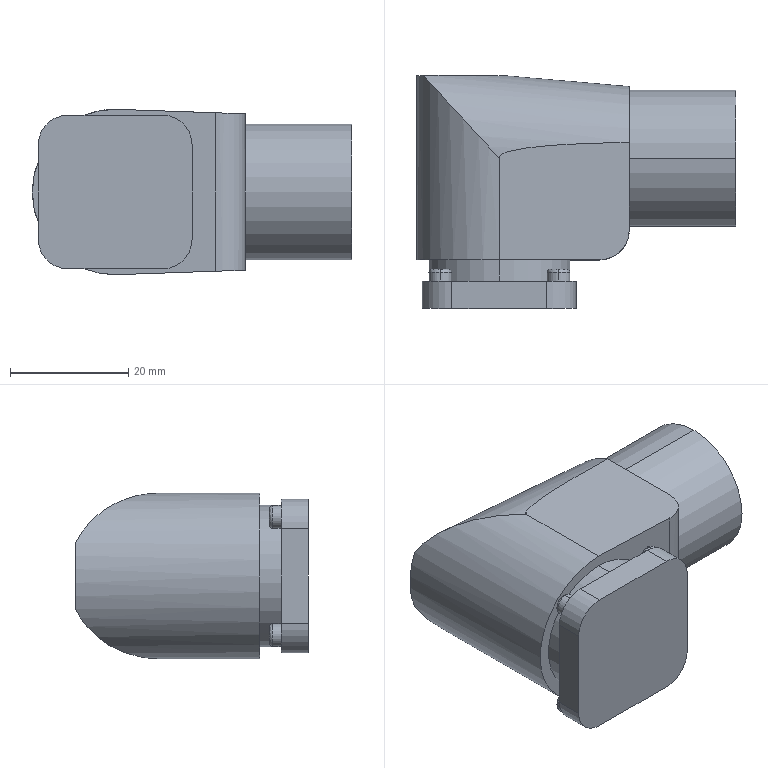Part | STEP file | _BMH070 Signalstecker gerade2 | 1 solid | 83 faces | box 54 x 39.4 x 28 mm | volume 35555 mm3 | cylinder 46 | plane 29 | spline 8 | commonest cylinder face diameters 1 x24 3.8 x8 10 x5 28 x3 19 x2 23 x2